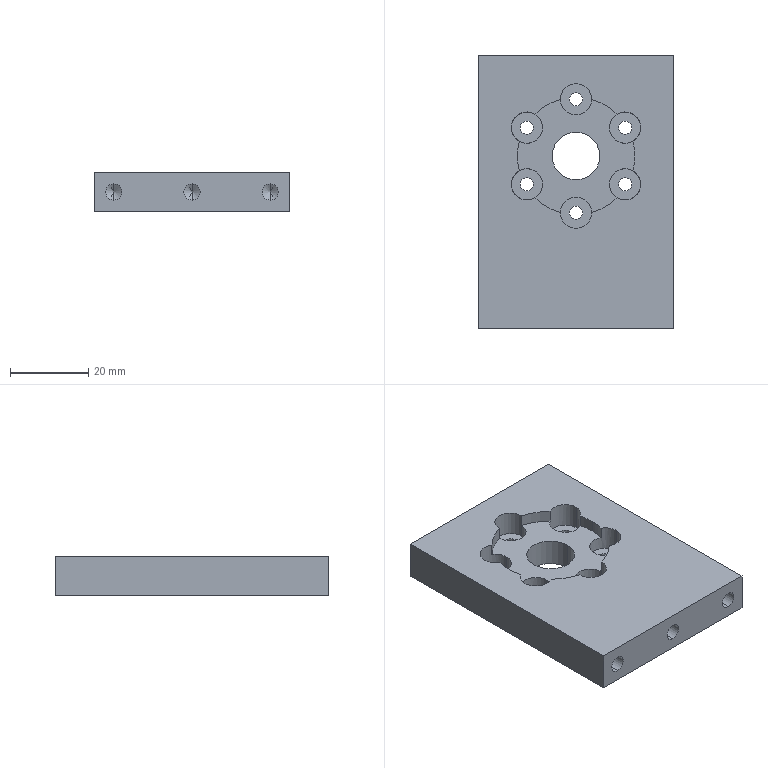Part | STEP file | 04-02-03 left bending cylinder mounting plate | 1 solid | 58 faces | box 50 x 70 x 10 mm | volume 29834 mm3 | cylinder 39 | plane 13 | cone 6 | commonest cylinder face diameters 3.4 x12 8 x12 30 x7 4.2 x6 12.2 x2